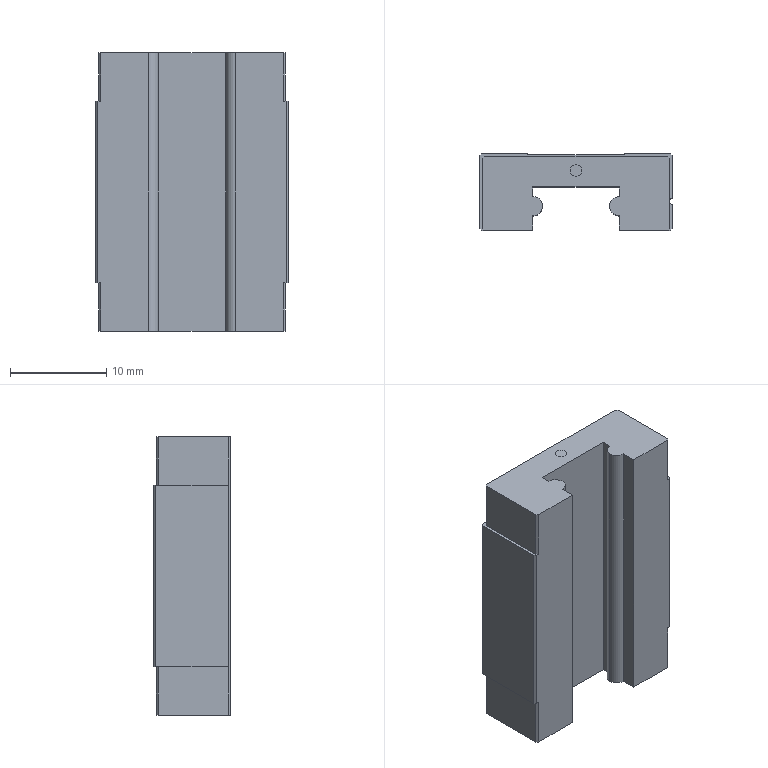Part | STEP file | 1 solid | 70 faces | box 20 x 8 x 29 mm | volume 3311 mm3 | plane 41 | cylinder 17 | cone 12 | commonest cylinder face diameters 3 x8 1.2 x4 2 x3 0.6 x2